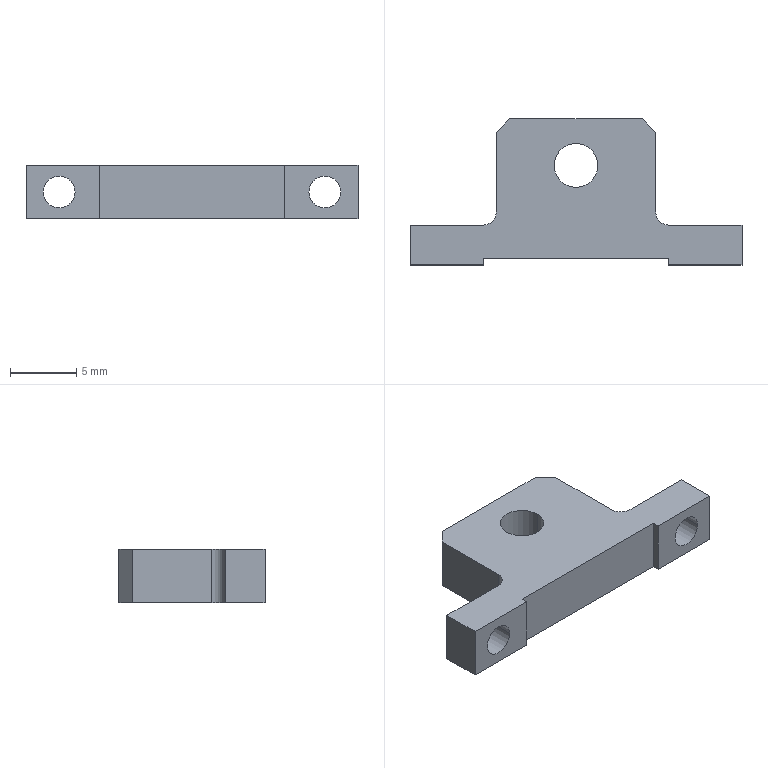Part | SolidWorks | features ICE 2, MoveFace 2, Chamfer 1, Extrusion 1, Fillet 1, HoleWzd 1 | 1 solid | 24 faces | box 25 x 11 x 4 mm | volume 592.362 mm3 | plane 16 | cylinder 8 | commonest cylinder face diameters 2.4 x4 2 x2 3.3 x2
STEP:
#1=CARTESIAN_POINT('',(25.2,0.,2.));
#2=VERTEX_POINT('',#1);
#3=CARTESIAN_POINT('',(22.8,0.,2.));
#4=VERTEX_POINT('',#3);
#5=CARTESIAN_POINT('',(24.,0.,2.));
#6=DIRECTION('',(0.,1.,0.));
#7=DIRECTION('',(-1.,0.,0.));
#8=AXIS2_PLACEMENT_3D('',#5,#6,#7);
#9=CIRCLE('',#8,1.2);
#10=EDGE_CURVE('',#2,#4,#9,.T.);
#11=ORIENTED_EDGE('',*,*,#10,.F.);
#12=CARTESIAN_POINT('',(25.2,3.,2.));
#13=VERTEX_POINT('',#12);
#14=CARTESIAN_POINT('',(25.2,0.,2.));
#15=DIRECTION('',(0.,1.,0.));
#16=VECTOR('',#15,1000.);
#17=LINE('',#14,#16);
#18=EDGE_CURVE('',#2,#13,#17,.T.);
#19=ORIENTED_EDGE('',*,*,#18,.T.);
#20=CARTESIAN_POINT('',(22.8,3.,2.));
#21=VERTEX_POINT('',#20);
#22=CARTESIAN_POINT('',(24.,3.,2.));
#23=DIRECTION('',(0.,-1.,0.));
#24=DIRECTION('',(1.,0.,0.));
#25=AXIS2_PLACEMENT_3D('',#22,#23,#24);
#26=CIRCLE('',#25,1.2);
#27=EDGE_CURVE('',#21,#13,#26,.T.);
#28=ORIENTED_EDGE('',*,*,#27,.F.);
#29=CARTESIAN_POINT('',(22.8,0.,2.));
#30=DIRECTION('',(0.,1.,0.));
#31=VECTOR('',#30,1000.);
#32=LINE('',#29,#31);
#33=EDGE_CURVE('',#4,#21,#32,.T.);
#34=ORIENTED_EDGE('',*,*,#33,.F.);
#35=EDGE_LOOP('',(#11,#19,#28,#34));
#36=FACE_OUTER_BOUND('',#35,.T.);
#37=CARTESIAN_POINT('',(24.,0.,2.));
#38=DIRECTION('',(0.,1.,0.));
#39=DIRECTION('',(-1.,0.,0.));
#40=AXIS2_PLACEMENT_3D('',#37,#38,#39);
#41=CYLINDRICAL_SURFACE('',#40,1.2);
#42=ADVANCED_FACE('',(#36),#41,.F.);
#43=CARTESIAN_POINT('',(5.2,0.,2.));
#44=VERTEX_POINT('',#43);
#45=CARTESIAN_POINT('',(2.8,0.,2.));
#46=VERTEX_POINT('',#45);
#47=CARTESIAN_POINT('',(4.,0.,2.));
#48=DIRECTION('',(0.,1.,0.));
#49=DIRECTION('',(-1.,0.,0.));
#50=AXIS2_PLACEMENT_3D('',#47,#48,#49);
#51=CIRCLE('',#50,1.2);
#52=EDGE_CURVE('',#44,#46,#51,.T.);
#53=ORIENTED_EDGE('',*,*,#52,.F.);
#54=CARTESIAN_POINT('',(5.2,3.,2.));
#55=VERTEX_POINT('',#54);
#56=CARTESIAN_POINT('',(5.2,0.,2.));
#57=DIRECTION('',(0.,1.,0.));
#58=VECTOR('',#57,1000.);
#59=LINE('',#56,#58);
#60=EDGE_CURVE('',#44,#55,#59,.T.);
#61=ORIENTED_EDGE('',*,*,#60,.T.);
#62=CARTESIAN_POINT('',(2.8,3.,2.));
#63=VERTEX_POINT('',#62);
#64=CARTESIAN_POINT('',(4.,3.,2.));
#65=DIRECTION('',(0.,-1.,0.));
#66=DIRECTION('',(1.,0.,0.));
#67=AXIS2_PLACEMENT_3D('',#64,#65,#66);
#68=CIRCLE('',#67,1.2);
#69=EDGE_CURVE('',#63,#55,#68,.T.);
#70=ORIENTED_EDGE('',*,*,#69,.F.);
#71=CARTESIAN_POINT('',(2.8,0.,2.));
#72=DIRECTION('',(0.,1.,0.));
#73=VECTOR('',#72,1000.);
#74=LINE('',#71,#73);
#75=EDGE_CURVE('',#46,#63,#74,.T.);
#76=ORIENTED_EDGE('',*,*,#75,.F.);
#77=EDGE_LOOP('',(#53,#61,#70,#76));
#78=FACE_OUTER_BOUND('',#77,.T.);
#79=CARTESIAN_POINT('',(4.,0.,2.));
#80=DIRECTION('',(0.,1.,0.));
#81=DIRECTION('',(-1.,0.,0.));
#82=AXIS2_PLACEMENT_3D('',#79,#80,#81);
#83=CYLINDRICAL_SURFACE('',#82,1.2);
#84=ADVANCED_FACE('',(#78),#83,.F.);
#85=CARTESIAN_POINT('',(12.35,7.5,0.));
#86=VERTEX_POINT('',#85);
#87=CARTESIAN_POINT('',(15.65,7.5,0.));
#88=VERTEX_POINT('',#87);
#89=CARTESIAN_POINT('',(14.,7.5,0.));
#90=DIRECTION('',(0.,0.,1.));
#91=DIRECTION('',(1.,0.,0.));
#92=AXIS2_PLACEMENT_3D('',#89,#90,#91);
#93=CIRCLE('',#92,1.65);
#94=EDGE_CURVE('',#86,#88,#93,.T.);
#95=ORIENTED_EDGE('',*,*,#94,.F.);
#96=CARTESIAN_POINT('',(12.35,7.5,4.));
#97=VERTEX_POINT('',#96);
#98=CARTESIAN_POINT('',(12.35,7.5,4.));
#99=DIRECTION('',(0.,0.,1.));
#100=VECTOR('',#99,1000.);
#101=LINE('',#98,#100);
#102=EDGE_CURVE('',#86,#97,#101,.T.);
#103=ORIENTED_EDGE('',*,*,#102,.T.);
#104=CARTESIAN_POINT('',(15.65,7.5,4.));
#105=VERTEX_POINT('',#104);
#106=CARTESIAN_POINT('',(14.,7.5,4.));
#107=DIRECTION('',(0.,0.,1.));
#108=DIRECTION('',(1.,0.,0.));
#109=AXIS2_PLACEMENT_3D('',#106,#107,#108);
#110=CIRCLE('',#109,1.65);
#111=EDGE_CURVE('',#97,#105,#110,.T.);
#112=ORIENTED_EDGE('',*,*,#111,.T.);
#113=CARTESIAN_POINT('',(15.65,7.5,4.));
#114=DIRECTION('',(0.,0.,1.));
#115=VECTOR('',#114,1000.);
#116=LINE('',#113,#115);
#117=EDGE_CURVE('',#88,#105,#116,.T.);
#118=ORIENTED_EDGE('',*,*,#117,.F.);
#119=EDGE_LOOP('',(#95,#103,#112,#118));
#120=FACE_OUTER_BOUND('',#119,.T.);
#121=CARTESIAN_POINT('',(14.,7.5,4.));
#122=DIRECTION('',(0.,0.,1.));
#123=DIRECTION('',(1.,0.,0.));
#124=AXIS2_PLACEMENT_3D('',#121,#122,#123);
#125=CYLINDRICAL_SURFACE('',#124,1.65);
#126=ADVANCED_FACE('',(#120),#125,.F.);
#127=CARTESIAN_POINT('',(4.,0.,2.));
#128=DIRECTION('',(0.,1.,0.));
#129=DIRECTION('',(-1.,0.,0.));
#130=AXIS2_PLACEMENT_3D('',#127,#128,#129);
#131=CIRCLE('',#130,1.2);
#132=EDGE_CURVE('',#46,#44,#131,.T.);
#133=ORIENTED_EDGE('',*,*,#132,.T.);
#134=ORIENTED_EDGE('',*,*,#52,.T.);
#135=EDGE_LOOP('',(#133,#134));
#136=FACE_BOUND('',#135,.T.);
#137=CARTESIAN_POINT('',(1.5,0.,0.));
#138=VERTEX_POINT('',#137);
#139=CARTESIAN_POINT('',(7.,0.,0.));
#140=VERTEX_POINT('',#139);
#141=CARTESIAN_POINT('',(0.,0.,0.));
#142=DIRECTION('',(1.,0.,0.));
#143=VECTOR('',#142,1000.);
#144=LINE('',#141,#143);
#145=EDGE_CURVE('',#138,#140,#144,.T.);
#146=ORIENTED_EDGE('',*,*,#145,.T.);
#147=CARTESIAN_POINT('',(7.,0.,4.));
#148=VERTEX_POINT('',#147);
#149=CARTESIAN_POINT('',(7.,0.,-6.));
#150=DIRECTION('',(0.,0.,1.));
#151=VECTOR('',#150,1000.);
#152=LINE('',#149,#151);
#153=EDGE_CURVE('',#140,#148,#152,.T.);
#154=ORIENTED_EDGE('',*,*,#153,.T.);
#155=CARTESIAN_POINT('',(1.5,0.,4.));
#156=VERTEX_POINT('',#155);
#157=CARTESIAN_POINT('',(0.,0.,4.));
#158=DIRECTION('',(1.,0.,0.));
#159=VECTOR('',#158,1000.);
#160=LINE('',#157,#159);
#161=EDGE_CURVE('',#156,#148,#160,.T.);
#162=ORIENTED_EDGE('',*,*,#161,.F.);
#163=CARTESIAN_POINT('',(1.5,0.,4.));
#164=DIRECTION('',(0.,0.,-1.));
#165=VECTOR('',#164,1000.);
#166=LINE('',#163,#165);
#167=EDGE_CURVE('',#156,#138,#166,.T.);
#168=ORIENTED_EDGE('',*,*,#167,.T.);
#169=EDGE_LOOP('',(#146,#154,#162,#168));
#170=FACE_OUTER_BOUND('',#169,.T.);
#171=CARTESIAN_POINT('',(0.,0.,4.));
#172=DIRECTION('',(0.,1.,0.));
#173=DIRECTION('',(0.,0.,1.));
#174=AXIS2_PLACEMENT_3D('',#171,#172,#173);
#175=PLANE('',#174);
#176=ADVANCED_FACE('',(#136,#170),#175,.F.);
#177=CARTESIAN_POINT('',(1.5,3.,0.));
#178=VERTEX_POINT('',#177);
#179=CARTESIAN_POINT('',(1.5,0.,0.));
#180=DIRECTION('',(0.,-1.,0.));
#181=VECTOR('',#180,1000.);
#182=LINE('',#179,#181);
#183=EDGE_CURVE('',#178,#138,#182,.T.);
#184=ORIENTED_EDGE('',*,*,#183,.T.);
#185=ORIENTED_EDGE('',*,*,#167,.F.);
#186=CARTESIAN_POINT('',(1.5,3.,4.));
#187=VERTEX_POINT('',#186);
#188=CARTESIAN_POINT('',(1.5,0.,4.));
#189=DIRECTION('',(0.,-1.,0.));
#190=VECTOR('',#189,1000.);
#191=LINE('',#188,#190);
#192=EDGE_CURVE('',#187,#156,#191,.T.);
#193=ORIENTED_EDGE('',*,*,#192,.F.);
#194=CARTESIAN_POINT('',(1.5,3.,4.));
#195=DIRECTION('',(0.,0.,-1.));
#196=VECTOR('',#195,1000.);
#197=LINE('',#194,#196);
#198=EDGE_CURVE('',#187,#178,#197,.T.);
#199=ORIENTED_EDGE('',*,*,#198,.T.);
#200=EDGE_LOOP('',(#184,#185,#193,#199));
#201=FACE_OUTER_BOUND('',#200,.T.);
#202=CARTESIAN_POINT('',(1.5,0.,4.));
#203=DIRECTION('',(1.,0.,0.));
#204=DIRECTION('',(0.,0.,-1.));
#205=AXIS2_PLACEMENT_3D('',#202,#203,#204);
#206=PLANE('',#205);
#207=ADVANCED_FACE('',(#201),#206,.F.);
#208=CARTESIAN_POINT('',(24.,0.,2.));
#209=DIRECTION('',(0.,1.,0.));
#210=DIRECTION('',(-1.,0.,0.));
#211=AXIS2_PLACEMENT_3D('',#208,#209,#210);
#212=CIRCLE('',#211,1.2);
#213=EDGE_CURVE('',#4,#2,#212,.T.);
#214=ORIENTED_EDGE('',*,*,#213,.T.);
#215=ORIENTED_EDGE('',*,*,#10,.T.);
#216=EDGE_LOOP('',(#214,#215));
#217=FACE_BOUND('',#216,.T.);
#218=CARTESIAN_POINT('',(21.,0.,4.));
#219=VERTEX_POINT('',#218);
#220=CARTESIAN_POINT('',(26.5,0.,4.));
#221=VERTEX_POINT('',#220);
#222=CARTESIAN_POINT('',(0.,0.,4.));
#223=DIRECTION('',(1.,0.,0.));
#224=VECTOR('',#223,1000.);
#225=LINE('',#222,#224);
#226=EDGE_CURVE('',#219,#221,#225,.T.);
#227=ORIENTED_EDGE('',*,*,#226,.F.);
#228=CARTESIAN_POINT('',(21.,0.,0.));
#229=VERTEX_POINT('',#228);
#230=CARTESIAN_POINT('',(21.,0.,-6.));
#231=DIRECTION('',(0.,0.,1.));
#232=VECTOR('',#231,1000.);
#233=LINE('',#230,#232);
#234=EDGE_CURVE('',#229,#219,#233,.T.);
#235=ORIENTED_EDGE('',*,*,#234,.F.);
#236=CARTESIAN_POINT('',(26.5,0.,0.));
#237=VERTEX_POINT('',#236);
#238=CARTESIAN_POINT('',(0.,0.,0.));
#239=DIRECTION('',(1.,0.,0.));
#240=VECTOR('',#239,1000.);
#241=LINE('',#238,#240);
#242=EDGE_CURVE('',#229,#237,#241,.T.);
#243=ORIENTED_EDGE('',*,*,#242,.T.);
#244=CARTESIAN_POINT('',(26.5,0.,4.));
#245=DIRECTION('',(0.,0.,-1.));
#246=VECTOR('',#245,1000.);
#247=LINE('',#244,#246);
#248=EDGE_CURVE('',#221,#237,#247,.T.);
#249=ORIENTED_EDGE('',*,*,#248,.F.);
#250=EDGE_LOOP('',(#227,#235,#243,#249));
#251=FACE_OUTER_BOUND('',#250,.T.);
#252=CARTESIAN_POINT('',(0.,0.,4.));
#253=DIRECTION('',(0.,1.,0.));
#254=DIRECTION('',(0.,0.,1.));
#255=AXIS2_PLACEMENT_3D('',#252,#253,#254);
#256=PLANE('',#255);
#257=ADVANCED_FACE('',(#217,#251),#256,.F.);
#258=CARTESIAN_POINT('',(26.5,3.,0.));
#259=VERTEX_POINT('',#258);
#260=CARTESIAN_POINT('',(26.5,0.,0.));
#261=DIRECTION('',(0.,1.,0.));
#262=VECTOR('',#261,1000.);
#263=LINE('',#260,#262);
#264=EDGE_CURVE('',#237,#259,#263,.T.);
#265=ORIENTED_EDGE('',*,*,#264,.T.);
#266=CARTESIAN_POINT('',(26.5,3.,4.));
#267=VERTEX_POINT('',#266);
#268=CARTESIAN_POINT('',(26.5,3.,4.));
#269=DIRECTION('',(0.,0.,-1.));
#270=VECTOR('',#269,1000.);
#271=LINE('',#268,#270);
#272=EDGE_CURVE('',#267,#259,#271,.T.);
#273=ORIENTED_EDGE('',*,*,#272,.F.);
#274=CARTESIAN_POINT('',(26.5,0.,4.));
#275=DIRECTION('',(0.,1.,0.));
#276=VECTOR('',#275,1000.);
#277=LINE('',#274,#276);
#278=EDGE_CURVE('',#221,#267,#277,.T.);
#279=ORIENTED_EDGE('',*,*,#278,.F.);
#280=ORIENTED_EDGE('',*,*,#248,.T.);
#281=EDGE_LOOP('',(#265,#273,#279,#280));
#282=FACE_OUTER_BOUND('',#281,.T.);
#283=CARTESIAN_POINT('',(26.5,0.,4.));
#284=DIRECTION('',(-1.,0.,0.));
#285=DIRECTION('',(0.,0.,1.));
#286=AXIS2_PLACEMENT_3D('',#283,#284,#285);
#287=PLANE('',#286);
#288=ADVANCED_FACE('',(#282),#287,.F.);
#289=ORIENTED_EDGE('',*,*,#27,.T.);
#290=CARTESIAN_POINT('',(24.,3.,2.));
#291=DIRECTION('',(0.,-1.,0.));
#292=DIRECTION('',(1.,0.,0.));
#293=AXIS2_PLACEMENT_3D('',#290,#291,#292);
#294=CIRCLE('',#293,1.2);
#295=EDGE_CURVE('',#13,#21,#294,.T.);
#296=ORIENTED_EDGE('',*,*,#295,.T.);
#297=EDGE_LOOP('',(#289,#296));
#298=FACE_BOUND('',#297,.T.);
#299=CARTESIAN_POINT('',(21.,3.,0.));
#300=VERTEX_POINT('',#299);
#301=CARTESIAN_POINT('',(28.,3.,0.));
#302=DIRECTION('',(-1.,0.,0.));
#303=VECTOR('',#302,1000.);
#304=LINE('',#301,#303);
#305=EDGE_CURVE('',#259,#300,#304,.T.);
#306=ORIENTED_EDGE('',*,*,#305,.T.);
#307=CARTESIAN_POINT('',(21.,3.,4.));
#308=VERTEX_POINT('',#307);
#309=CARTESIAN_POINT('',(21.,3.,4.));
#310=DIRECTION('',(0.,0.,1.));
#311=VECTOR('',#310,1000.);
#312=LINE('',#309,#311);
#313=EDGE_CURVE('',#300,#308,#312,.T.);
#314=ORIENTED_EDGE('',*,*,#313,.T.);
#315=CARTESIAN_POINT('',(28.,3.,4.));
#316=DIRECTION('',(-1.,0.,0.));
#317=VECTOR('',#316,1000.);
#318=LINE('',#315,#317);
#319=EDGE_CURVE('',#267,#308,#318,.T.);
#320=ORIENTED_EDGE('',*,*,#319,.F.);
#321=ORIENTED_EDGE('',*,*,#272,.T.);
#322=EDGE_LOOP('',(#306,#314,#320,#321));
#323=FACE_OUTER_BOUND('',#322,.T.);
#324=CARTESIAN_POINT('',(28.,3.,4.));
#325=DIRECTION('',(0.,-1.,0.));
#326=DIRECTION('',(1.,0.,0.));
#327=AXIS2_PLACEMENT_3D('',#324,#325,#326);
#328=PLANE('',#327);
#329=ADVANCED_FACE('',(#298,#323),#328,.F.);
#330=CARTESIAN_POINT('',(20.,4.,0.));
#331=VERTEX_POINT('',#330);
#332=CARTESIAN_POINT('',(20.,10.,0.));
#333=VERTEX_POINT('',#332);
#334=CARTESIAN_POINT('',(20.,3.,0.));
#335=DIRECTION('',(0.,1.,0.));
#336=VECTOR('',#335,1000.);
#337=LINE('',#334,#336);
#338=EDGE_CURVE('',#331,#333,#337,.T.);
#339=ORIENTED_EDGE('',*,*,#338,.T.);
#340=CARTESIAN_POINT('',(20.,10.,4.));
#341=VERTEX_POINT('',#340);
#342=CARTESIAN_POINT('',(20.,10.,4.));
#343=DIRECTION('',(0.,0.,1.));
#344=VECTOR('',#343,1000.);
#345=LINE('',#342,#344);
#346=EDGE_CURVE('',#333,#341,#345,.T.);
#347=ORIENTED_EDGE('',*,*,#346,.T.);
#348=CARTESIAN_POINT('',(20.,4.,4.));
#349=VERTEX_POINT('',#348);
#350=CARTESIAN_POINT('',(20.,3.,4.));
#351=DIRECTION('',(0.,1.,0.));
#352=VECTOR('',#351,1000.);
#353=LINE('',#350,#352);
#354=EDGE_CURVE('',#349,#341,#353,.T.);
#355=ORIENTED_EDGE('',*,*,#354,.F.);
#356=CARTESIAN_POINT('',(20.,4.,0.));
#357=DIRECTION('',(0.,0.,-1.));
#358=VECTOR('',#357,1000.);
#359=LINE('',#356,#358);
#360=EDGE_CURVE('',#349,#331,#359,.T.);
#361=ORIENTED_EDGE('',*,*,#360,.T.);
#362=EDGE_LOOP('',(#339,#347,#355,#361));
#363=FACE_OUTER_BOUND('',#362,.T.);
#364=CARTESIAN_POINT('',(20.,3.,4.));
#365=DIRECTION('',(-1.,0.,0.));
#366=DIRECTION('',(0.,0.,1.));
#367=AXIS2_PLACEMENT_3D('',#364,#365,#366);
#368=PLANE('',#367);
#369=ADVANCED_FACE('',(#363),#368,.F.);
#370=CARTESIAN_POINT('',(19.,11.,0.));
#371=VERTEX_POINT('',#370);
#372=CARTESIAN_POINT('',(9.,11.,0.));
#373=VERTEX_POINT('',#372);
#374=CARTESIAN_POINT('',(20.,11.,0.));
#375=DIRECTION('',(-1.,0.,0.));
#376=VECTOR('',#375,1000.);
#377=LINE('',#374,#376);
#378=EDGE_CURVE('',#371,#373,#377,.T.);
#379=ORIENTED_EDGE('',*,*,#378,.T.);
#380=CARTESIAN_POINT('',(9.,11.,4.));
#381=VERTEX_POINT('',#380);
#382=CARTESIAN_POINT('',(9.,11.,4.));
#383=DIRECTION('',(0.,0.,1.));
#384=VECTOR('',#383,1000.);
#385=LINE('',#382,#384);
#386=EDGE_CURVE('',#373,#381,#385,.T.);
#387=ORIENTED_EDGE('',*,*,#386,.T.);
#388=CARTESIAN_POINT('',(19.,11.,4.));
#389=VERTEX_POINT('',#388);
#390=CARTESIAN_POINT('',(20.,11.,4.));
#391=DIRECTION('',(-1.,0.,0.));
#392=VECTOR('',#391,1000.);
#393=LINE('',#390,#392);
#394=EDGE_CURVE('',#389,#381,#393,.T.);
#395=ORIENTED_EDGE('',*,*,#394,.F.);
#396=CARTESIAN_POINT('',(19.,11.,4.));
#397=DIRECTION('',(0.,0.,-1.));
#398=VECTOR('',#397,1000.);
#399=LINE('',#396,#398);
#400=EDGE_CURVE('',#389,#371,#399,.T.);
#401=ORIENTED_EDGE('',*,*,#400,.T.);
#402=EDGE_LOOP('',(#379,#387,#395,#401));
#403=FACE_OUTER_BOUND('',#402,.T.);
#404=CARTESIAN_POINT('',(20.,11.,4.));
#405=DIRECTION('',(0.,-1.,0.));
#406=DIRECTION('',(1.,0.,0.));
#407=AXIS2_PLACEMENT_3D('',#404,#405,#406);
#408=PLANE('',#407);
#409=ADVANCED_FACE('',(#403),#408,.F.);
#410=CARTESIAN_POINT('',(8.,10.,4.));
#411=VERTEX_POINT('',#410);
#412=CARTESIAN_POINT('',(8.,4.,4.));
#413=VERTEX_POINT('',#412);
#414=CARTESIAN_POINT('',(8.,3.,4.));
#415=DIRECTION('',(0.,-1.,0.));
#416=VECTOR('',#415,1000.);
#417=LINE('',#414,#416);
#418=EDGE_CURVE('',#411,#413,#417,.T.);
#419=ORIENTED_EDGE('',*,*,#418,.F.);
#420=CARTESIAN_POINT('',(8.,10.,0.));
#421=VERTEX_POINT('',#420);
#422=CARTESIAN_POINT('',(8.,10.,4.));
#423=DIRECTION('',(0.,0.,-1.));
#424=VECTOR('',#423,1000.);
#425=LINE('',#422,#424);
#426=EDGE_CURVE('',#411,#421,#425,.T.);
#427=ORIENTED_EDGE('',*,*,#426,.T.);
#428=CARTESIAN_POINT('',(8.,4.,0.));
#429=VERTEX_POINT('',#428);
#430=CARTESIAN_POINT('',(8.,3.,0.));
#431=DIRECTION('',(0.,-1.,0.));
#432=VECTOR('',#431,1000.);
#433=LINE('',#430,#432);
#434=EDGE_CURVE('',#421,#429,#433,.T.);
#435=ORIENTED_EDGE('',*,*,#434,.T.);
#436=CARTESIAN_POINT('',(8.,4.,4.));
#437=DIRECTION('',(0.,0.,1.));
#438=VECTOR('',#437,1000.);
#439=LINE('',#436,#438);
#440=EDGE_CURVE('',#429,#413,#439,.T.);
#441=ORIENTED_EDGE('',*,*,#440,.T.);
#442=EDGE_LOOP('',(#419,#427,#435,#441));
#443=FACE_OUTER_BOUND('',#442,.T.);
#444=CARTESIAN_POINT('',(8.,3.,4.));
#445=DIRECTION('',(1.,0.,0.));
#446=DIRECTION('',(0.,0.,-1.));
#447=AXIS2_PLACEMENT_3D('',#444,#445,#446);
#448=PLANE('',#447);
#449=ADVANCED_FACE('',(#443),#448,.F.);
#450=ORIENTED_EDGE('',*,*,#69,.T.);
#451=CARTESIAN_POINT('',(4.,3.,2.));
#452=DIRECTION('',(0.,-1.,0.));
#453=DIRECTION('',(1.,0.,0.));
#454=AXIS2_PLACEMENT_3D('',#451,#452,#453);
#455=CIRCLE('',#454,1.2);
#456=EDGE_CURVE('',#55,#63,#455,.T.);
#457=ORIENTED_EDGE('',*,*,#456,.T.);
#458=EDGE_LOOP('',(#450,#457));
#459=FACE_BOUND('',#458,.T.);
#460=CARTESIAN_POINT('',(7.,3.,4.));
#461=VERTEX_POINT('',#460);
#462=CARTESIAN_POINT('',(0.,3.,4.));
#463=DIRECTION('',(-1.,0.,0.));
#464=VECTOR('',#463,1000.);
#465=LINE('',#462,#464);
#466=EDGE_CURVE('',#461,#187,#465,.T.);
#467=ORIENTED_EDGE('',*,*,#466,.F.);
#468=CARTESIAN_POINT('',(7.,3.,0.));
#469=VERTEX_POINT('',#468);
#470=CARTESIAN_POINT('',(7.,3.,0.));
#471=DIRECTION('',(0.,0.,-1.));
#472=VECTOR('',#471,1000.);
#473=LINE('',#470,#472);
#474=EDGE_CURVE('',#461,#469,#473,.T.);
#475=ORIENTED_EDGE('',*,*,#474,.T.);
#476=CARTESIAN_POINT('',(0.,3.,0.));
#477=DIRECTION('',(-1.,0.,0.));
#478=VECTOR('',#477,1000.);
#479=LINE('',#476,#478);
#480=EDGE_CURVE('',#469,#178,#479,.T.);
#481=ORIENTED_EDGE('',*,*,#480,.T.);
#482=ORIENTED_EDGE('',*,*,#198,.F.);
#483=EDGE_LOOP('',(#467,#475,#481,#482));
#484=FACE_OUTER_BOUND('',#483,.T.);
#485=CARTESIAN_POINT('',(0.,3.,4.));
#486=DIRECTION('',(0.,-1.,0.));
#487=DIRECTION('',(1.,0.,0.));
#488=AXIS2_PLACEMENT_3D('',#485,#486,#487);
#489=PLANE('',#488);
#490=ADVANCED_FACE('',(#459,#484),#489,.F.);
#491=CARTESIAN_POINT('',(14.,7.5,4.));
#492=DIRECTION('',(0.,0.,1.));
#493=DIRECTION('',(1.,0.,0.));
#494=AXIS2_PLACEMENT_3D('',#491,#492,#493);
#495=CIRCLE('',#494,1.65);
#496=EDGE_CURVE('',#105,#97,#495,.T.);
#497=ORIENTED_EDGE('',*,*,#496,.F.);
#498=ORIENTED_EDGE('',*,*,#111,.F.);
#499=EDGE_LOOP('',(#497,#498));
#500=FACE_BOUND('',#499,.T.);
#501=ORIENTED_EDGE('',*,*,#161,.T.);
#502=CARTESIAN_POINT('',(7.,0.5,4.));
#503=VERTEX_POINT('',#502);
#504=CARTESIAN_POINT('',(7.,0.,4.));
#505=DIRECTION('',(0.,-1.,0.));
#506=VECTOR('',#505,1000.);
#507=LINE('',#504,#506);
#508=EDGE_CURVE('',#503,#148,#507,.T.);
#509=ORIENTED_EDGE('',*,*,#508,.F.);
#510=CARTESIAN_POINT('',(21.,0.5,4.));
#511=VERTEX_POINT('',#510);
#512=CARTESIAN_POINT('',(7.,0.5,4.));
#513=DIRECTION('',(-1.,0.,0.));
#514=VECTOR('',#513,1000.);
#515=LINE('',#512,#514);
#516=EDGE_CURVE('',#511,#503,#515,.T.);
#517=ORIENTED_EDGE('',*,*,#516,.F.);
#518=CARTESIAN_POINT('',(21.,0.5,4.));
#519=DIRECTION('',(0.,1.,0.));
#520=VECTOR('',#519,1000.);
#521=LINE('',#518,#520);
#522=EDGE_CURVE('',#219,#511,#521,.T.);
#523=ORIENTED_EDGE('',*,*,#522,.F.);
#524=ORIENTED_EDGE('',*,*,#226,.T.);
#525=ORIENTED_EDGE('',*,*,#278,.T.);
#526=ORIENTED_EDGE('',*,*,#319,.T.);
#527=CARTESIAN_POINT('',(21.,4.,4.));
#528=DIRECTION('',(0.,0.,-1.));
#529=DIRECTION('',(-1.,0.,0.));
#530=AXIS2_PLACEMENT_3D('',#527,#528,#529);
#531=CIRCLE('',#530,1.);
#532=EDGE_CURVE('',#308,#349,#531,.T.);
#533=ORIENTED_EDGE('',*,*,#532,.T.);
#534=ORIENTED_EDGE('',*,*,#354,.T.);
#535=CARTESIAN_POINT('',(19.,11.,4.));
#536=DIRECTION('',(-0.7071,0.7071,0.));
#537=VECTOR('',#536,1000.);
#538=LINE('',#535,#537);
#539=EDGE_CURVE('',#341,#389,#538,.T.);
#540=ORIENTED_EDGE('',*,*,#539,.T.);
#541=ORIENTED_EDGE('',*,*,#394,.T.);
#542=CARTESIAN_POINT('',(8.,10.,4.));
#543=DIRECTION('',(-0.7071,-0.7071,0.));
#544=VECTOR('',#543,1000.);
#545=LINE('',#542,#544);
#546=EDGE_CURVE('',#381,#411,#545,.T.);
#547=ORIENTED_EDGE('',*,*,#546,.T.);
#548=ORIENTED_EDGE('',*,*,#418,.T.);
#549=CARTESIAN_POINT('',(7.,4.,4.));
#550=DIRECTION('',(0.,0.,-1.));
#551=DIRECTION('',(-1.,0.,0.));
#552=AXIS2_PLACEMENT_3D('',#549,#550,#551);
#553=CIRCLE('',#552,1.);
#554=EDGE_CURVE('',#413,#461,#553,.T.);
#555=ORIENTED_EDGE('',*,*,#554,.T.);
#556=ORIENTED_EDGE('',*,*,#466,.T.);
#557=ORIENTED_EDGE('',*,*,#192,.T.);
#558=EDGE_LOOP('',(#501,#509,#517,#523,#524,#525,#526,#533,#534,#540,#541,#547,#548,#555,#556,#557));
#559=FACE_OUTER_BOUND('',#558,.T.);
#560=CARTESIAN_POINT('',(0.,0.,4.));
#561=DIRECTION('',(0.,0.,-1.));
#562=DIRECTION('',(-1.,0.,0.));
#563=AXIS2_PLACEMENT_3D('',#560,#561,#562);
#564=PLANE('',#563);
#565=ADVANCED_FACE('',(#500,#559),#564,.F.);
#566=CARTESIAN_POINT('',(7.,0.5,0.));
#567=VERTEX_POINT('',#566);
#568=CARTESIAN_POINT('',(7.,0.,0.));
#569=DIRECTION('',(0.,1.,0.));
#570=VECTOR('',#569,1000.);
#571=LINE('',#568,#570);
#572=EDGE_CURVE('',#140,#567,#571,.T.);
#573=ORIENTED_EDGE('',*,*,#572,.F.);
#574=ORIENTED_EDGE('',*,*,#145,.F.);
#575=ORIENTED_EDGE('',*,*,#183,.F.);
#576=ORIENTED_EDGE('',*,*,#480,.F.);
#577=CARTESIAN_POINT('',(7.,4.,0.));
#578=DIRECTION('',(0.,0.,1.));
#579=DIRECTION('',(-1.,0.,0.));
#580=AXIS2_PLACEMENT_3D('',#577,#578,#579);
#581=CIRCLE('',#580,1.);
#582=EDGE_CURVE('',#469,#429,#581,.T.);
#583=ORIENTED_EDGE('',*,*,#582,.T.);
#584=ORIENTED_EDGE('',*,*,#434,.F.);
#585=CARTESIAN_POINT('',(-1.,1.,0.));
#586=DIRECTION('',(0.7071,0.7071,0.));
#587=VECTOR('',#586,1000.);
#588=LINE('',#585,#587);
#589=EDGE_CURVE('',#421,#373,#588,.T.);
#590=ORIENTED_EDGE('',*,*,#589,.T.);
#591=ORIENTED_EDGE('',*,*,#378,.F.);
#592=CARTESIAN_POINT('',(15.,15.,0.));
#593=DIRECTION('',(0.7071,-0.7071,0.));
#594=VECTOR('',#593,1000.);
#595=LINE('',#592,#594);
#596=EDGE_CURVE('',#371,#333,#595,.T.);
#597=ORIENTED_EDGE('',*,*,#596,.T.);
#598=ORIENTED_EDGE('',*,*,#338,.F.);
#599=CARTESIAN_POINT('',(21.,4.,0.));
#600=DIRECTION('',(0.,0.,1.));
#601=DIRECTION('',(-1.,0.,0.));
#602=AXIS2_PLACEMENT_3D('',#599,#600,#601);
#603=CIRCLE('',#602,1.);
#604=EDGE_CURVE('',#331,#300,#603,.T.);
#605=ORIENTED_EDGE('',*,*,#604,.T.);
#606=ORIENTED_EDGE('',*,*,#305,.F.);
#607=ORIENTED_EDGE('',*,*,#264,.F.);
#608=ORIENTED_EDGE('',*,*,#242,.F.);
#609=CARTESIAN_POINT('',(21.,0.5,0.));
#610=VERTEX_POINT('',#609);
#611=CARTESIAN_POINT('',(21.,0.,0.));
#612=DIRECTION('',(0.,-1.,0.));
#613=VECTOR('',#612,1000.);
#614=LINE('',#611,#613);
#615=EDGE_CURVE('',#610,#229,#614,.T.);
#616=ORIENTED_EDGE('',*,*,#615,.F.);
#617=CARTESIAN_POINT('',(0.,0.5,0.));
#618=DIRECTION('',(1.,0.,0.));
#619=VECTOR('',#618,1000.);
#620=LINE('',#617,#619);
#621=EDGE_CURVE('',#567,#610,#620,.T.);
#622=ORIENTED_EDGE('',*,*,#621,.F.);
#623=EDGE_LOOP('',(#573,#574,#575,#576,#583,#584,#590,#591,#597,#598,#605,#606,#607,#608,#616,#622));
#624=FACE_OUTER_BOUND('',#623,.T.);
#625=CARTESIAN_POINT('',(14.,7.5,0.));
#626=DIRECTION('',(0.,0.,1.));
#627=DIRECTION('',(1.,0.,0.));
#628=AXIS2_PLACEMENT_3D('',#625,#626,#627);
#629=CIRCLE('',#628,1.65);
#630=EDGE_CURVE('',#88,#86,#629,.T.);
#631=ORIENTED_EDGE('',*,*,#630,.T.);
#632=ORIENTED_EDGE('',*,*,#94,.T.);
#633=EDGE_LOOP('',(#631,#632));
#634=FACE_BOUND('',#633,.T.);
#635=CARTESIAN_POINT('',(0.,0.,0.));
#636=DIRECTION('',(0.,0.,-1.));
#637=DIRECTION('',(-1.,0.,0.));
#638=AXIS2_PLACEMENT_3D('',#635,#636,#637);
#639=PLANE('',#638);
#640=ADVANCED_FACE('',(#624,#634),#639,.T.);
#641=ORIENTED_EDGE('',*,*,#102,.F.);
#642=ORIENTED_EDGE('',*,*,#630,.F.);
#643=ORIENTED_EDGE('',*,*,#117,.T.);
#644=ORIENTED_EDGE('',*,*,#496,.T.);
#645=EDGE_LOOP('',(#641,#642,#643,#644));
#646=FACE_OUTER_BOUND('',#645,.T.);
#647=CARTESIAN_POINT('',(14.,7.5,4.));
#648=DIRECTION('',(0.,0.,1.));
#649=DIRECTION('',(1.,0.,0.));
#650=AXIS2_PLACEMENT_3D('',#647,#648,#649);
#651=CYLINDRICAL_SURFACE('',#650,1.65);
#652=ADVANCED_FACE('',(#646),#651,.F.);
#653=ORIENTED_EDGE('',*,*,#60,.F.);
#654=ORIENTED_EDGE('',*,*,#132,.F.);
#655=ORIENTED_EDGE('',*,*,#75,.T.);
#656=ORIENTED_EDGE('',*,*,#456,.F.);
#657=EDGE_LOOP('',(#653,#654,#655,#656));
#658=FACE_OUTER_BOUND('',#657,.T.);
#659=CARTESIAN_POINT('',(4.,0.,2.));
#660=DIRECTION('',(0.,1.,0.));
#661=DIRECTION('',(-1.,0.,0.));
#662=AXIS2_PLACEMENT_3D('',#659,#660,#661);
#663=CYLINDRICAL_SURFACE('',#662,1.2);
#664=ADVANCED_FACE('',(#658),#663,.F.);
#665=ORIENTED_EDGE('',*,*,#18,.F.);
#666=ORIENTED_EDGE('',*,*,#213,.F.);
#667=ORIENTED_EDGE('',*,*,#33,.T.);
#668=ORIENTED_EDGE('',*,*,#295,.F.);
#669=EDGE_LOOP('',(#665,#666,#667,#668));
#670=FACE_OUTER_BOUND('',#669,.T.);
#671=CARTESIAN_POINT('',(24.,0.,2.));
#672=DIRECTION('',(0.,1.,0.));
#673=DIRECTION('',(-1.,0.,0.));
#674=AXIS2_PLACEMENT_3D('',#671,#672,#673);
#675=CYLINDRICAL_SURFACE('',#674,1.2);
#676=ADVANCED_FACE('',(#670),#675,.F.);
#677=ORIENTED_EDGE('',*,*,#532,.F.);
#678=ORIENTED_EDGE('',*,*,#313,.F.);
#679=ORIENTED_EDGE('',*,*,#604,.F.);
#680=ORIENTED_EDGE('',*,*,#360,.F.);
#681=EDGE_LOOP('',(#677,#678,#679,#680));
#682=FACE_OUTER_BOUND('',#681,.T.);
#683=CARTESIAN_POINT('',(21.,4.,4.));
#684=DIRECTION('',(0.,0.,1.));
#685=DIRECTION('',(1.,0.,0.));
#686=AXIS2_PLACEMENT_3D('',#683,#684,#685);
#687=CYLINDRICAL_SURFACE('',#686,1.);
#688=ADVANCED_FACE('',(#682),#687,.F.);
#689=ORIENTED_EDGE('',*,*,#554,.F.);
#690=ORIENTED_EDGE('',*,*,#440,.F.);
#691=ORIENTED_EDGE('',*,*,#582,.F.);
#692=ORIENTED_EDGE('',*,*,#474,.F.);
#693=EDGE_LOOP('',(#689,#690,#691,#692));
#694=FACE_OUTER_BOUND('',#693,.T.);
#695=CARTESIAN_POINT('',(7.,4.,4.));
#696=DIRECTION('',(0.,0.,1.));
#697=DIRECTION('',(1.,0.,0.));
#698=AXIS2_PLACEMENT_3D('',#695,#696,#697);
#699=CYLINDRICAL_SURFACE('',#698,1.);
#700=ADVANCED_FACE('',(#694),#699,.F.);
#701=ORIENTED_EDGE('',*,*,#546,.F.);
#702=ORIENTED_EDGE('',*,*,#386,.F.);
#703=ORIENTED_EDGE('',*,*,#589,.F.);
#704=ORIENTED_EDGE('',*,*,#426,.F.);
#705=EDGE_LOOP('',(#701,#702,#703,#704));
#706=FACE_OUTER_BOUND('',#705,.T.);
#707=CARTESIAN_POINT('',(8.,10.,4.));
#708=DIRECTION('',(0.7071,-0.7071,0.));
#709=DIRECTION('',(0.,0.,-1.));
#710=AXIS2_PLACEMENT_3D('',#707,#708,#709);
#711=PLANE('',#710);
#712=ADVANCED_FACE('',(#706),#711,.F.);
#713=ORIENTED_EDGE('',*,*,#539,.F.);
#714=ORIENTED_EDGE('',*,*,#346,.F.);
#715=ORIENTED_EDGE('',*,*,#596,.F.);
#716=ORIENTED_EDGE('',*,*,#400,.F.);
#717=EDGE_LOOP('',(#713,#714,#715,#716));
#718=FACE_OUTER_BOUND('',#717,.T.);
#719=CARTESIAN_POINT('',(19.,11.,4.));
#720=DIRECTION('',(-0.7071,-0.7071,0.));
#721=DIRECTION('',(0.,0.,-1.));
#722=AXIS2_PLACEMENT_3D('',#719,#720,#721);
#723=PLANE('',#722);
#724=ADVANCED_FACE('',(#718),#723,.F.);
#725=ORIENTED_EDGE('',*,*,#572,.T.);
#726=CARTESIAN_POINT('',(7.,0.5,-6.));
#727=DIRECTION('',(0.,0.,1.));
#728=VECTOR('',#727,1000.);
#729=LINE('',#726,#728);
#730=EDGE_CURVE('',#567,#503,#729,.T.);
#731=ORIENTED_EDGE('',*,*,#730,.T.);
#732=ORIENTED_EDGE('',*,*,#508,.T.);
#733=ORIENTED_EDGE('',*,*,#153,.F.);
#734=EDGE_LOOP('',(#725,#731,#732,#733));
#735=FACE_OUTER_BOUND('',#734,.T.);
#736=CARTESIAN_POINT('',(7.,0.,-6.));
#737=DIRECTION('',(-1.,0.,0.));
#738=DIRECTION('',(0.,-1.,0.));
#739=AXIS2_PLACEMENT_3D('',#736,#737,#738);
#740=PLANE('',#739);
#741=ADVANCED_FACE('',(#735),#740,.F.);
#742=ORIENTED_EDGE('',*,*,#621,.T.);
#743=CARTESIAN_POINT('',(21.,0.5,-6.));
#744=DIRECTION('',(0.,0.,1.));
#745=VECTOR('',#744,1000.);
#746=LINE('',#743,#745);
#747=EDGE_CURVE('',#610,#511,#746,.T.);
#748=ORIENTED_EDGE('',*,*,#747,.T.);
#749=ORIENTED_EDGE('',*,*,#516,.T.);
#750=ORIENTED_EDGE('',*,*,#730,.F.);
#751=EDGE_LOOP('',(#742,#748,#749,#750));
#752=FACE_OUTER_BOUND('',#751,.T.);
#753=CARTESIAN_POINT('',(7.,0.5,-6.));
#754=DIRECTION('',(0.,1.,0.));
#755=DIRECTION('',(0.,0.,1.));
#756=AXIS2_PLACEMENT_3D('',#753,#754,#755);
#757=PLANE('',#756);
#758=ADVANCED_FACE('',(#752),#757,.F.);
#759=ORIENTED_EDGE('',*,*,#615,.T.);
#760=ORIENTED_EDGE('',*,*,#234,.T.);
#761=ORIENTED_EDGE('',*,*,#522,.T.);
#762=ORIENTED_EDGE('',*,*,#747,.F.);
#763=EDGE_LOOP('',(#759,#760,#761,#762));
#764=FACE_OUTER_BOUND('',#763,.T.);
#765=CARTESIAN_POINT('',(21.,0.5,-6.));
#766=DIRECTION('',(1.,0.,0.));
#767=DIRECTION('',(0.,0.,-1.));
#768=AXIS2_PLACEMENT_3D('',#765,#766,#767);
#769=PLANE('',#768);
#770=ADVANCED_FACE('',(#764),#769,.F.);
#771=CLOSED_SHELL('',(#42,#84,#126,#176,#207,#257,#288,#329,#369,#409,#449,#490,#565,#640,#652,#664,#676,#688,#700,#712,#724,#741,#758,#770));
#772=MANIFOLD_SOLID_BREP('',#771);
#773=CARTESIAN_POINT('',(0.,0.,0.));
#774=DIRECTION('',(0.,0.,1.));
#775=DIRECTION('',(1.,0.,0.));
#776=AXIS2_PLACEMENT_3D('',#773,#774,#775);
#777=(LENGTH_UNIT()NAMED_UNIT(*)SI_UNIT(.MILLI.,.METRE.));
#778=UNCERTAINTY_MEASURE_WITH_UNIT(LENGTH_MEASURE(0.00001),#777,'','');
#779=(NAMED_UNIT(*)PLANE_ANGLE_UNIT()SI_UNIT($,.RADIAN.));
#780=(NAMED_UNIT(*)SI_UNIT($,.STERADIAN.)SOLID_ANGLE_UNIT());
#781=(GEOMETRIC_REPRESENTATION_CONTEXT(3)GLOBAL_UNCERTAINTY_ASSIGNED_CONTEXT((#778))GLOBAL_UNIT_ASSIGNED_CONTEXT((#777,#779,#780))REPRESENTATION_CONTEXT('',''));
#782=ADVANCED_BREP_SHAPE_REPRESENTATION('',(#772,#776),#781);